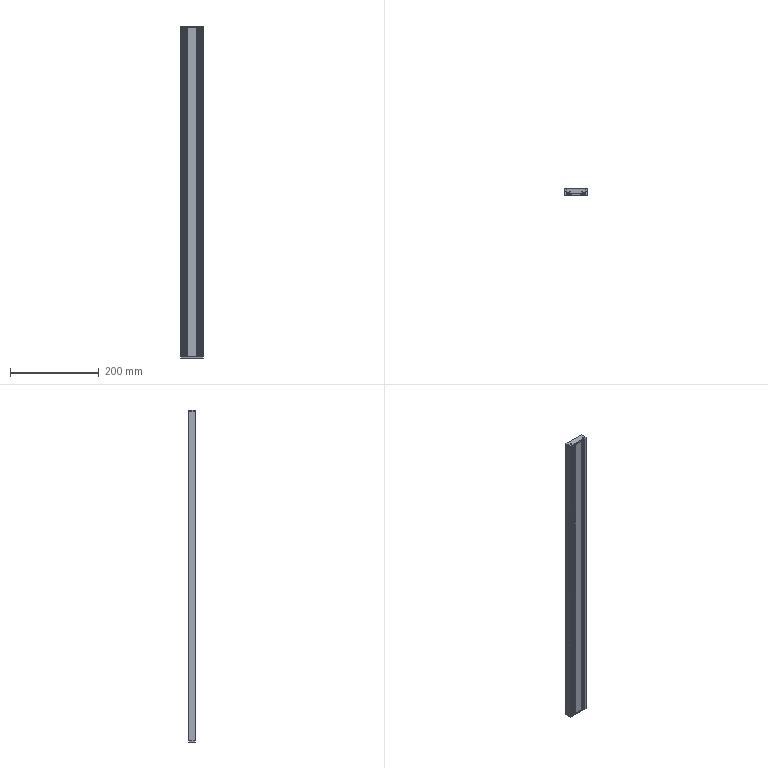Part | SolidWorks | features ICE 3, Fillet 2, Extrusion 1, MirrorSolid 1 | 3 solids | 294 faces | box 50 x 15 x 750 mm | volume 379215 mm3 | plane 245 | cylinder 49 | commonest cylinder face diameters 1 x12 2 x8 3.5 x8 0.4 x4 1.1 x4 5.948 x4